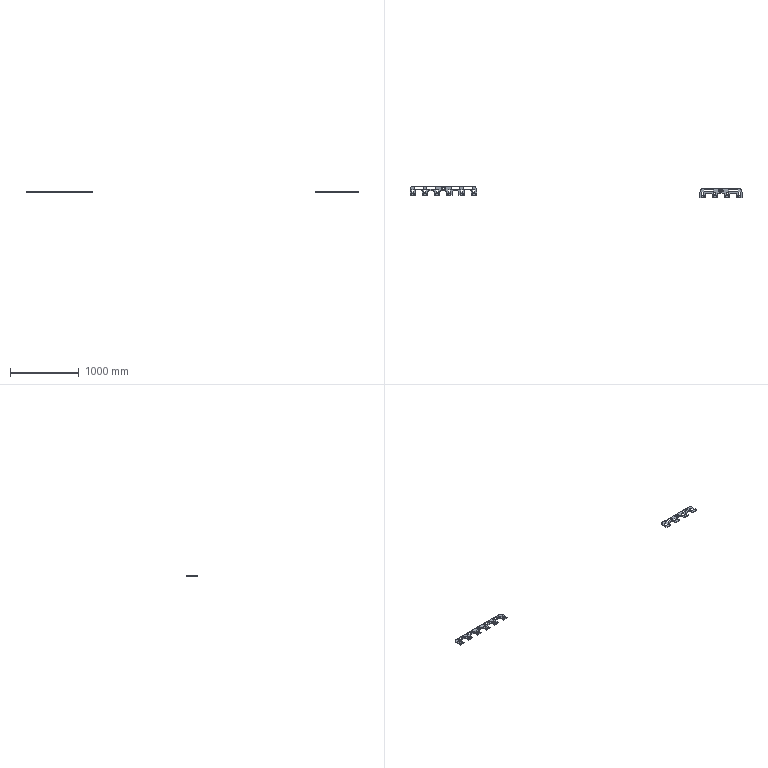NC program | NX | posted with a generic post | part box 4825 x 168.213 x 13 mm
Lines 6552 to 7588 of 14244:
(HOLE_MILLING_COPY , TOOL : D6)
N13054 T06 M6
N13056 G54
N13058 G17 G0 G90 X472.685 Y58.869 S9500 M3
N13060 G43 Z30. H6
N13062 Z0.5
N13064 G94 G3 X473.185 Y58.369 R0.5 F1400.
N13066 X473.685 Y58.869 R0.5
N13068 X473.685 Y58.869 Z0. I-1. J0.
N13070 X473.685 Y58.869 Z-0.5 I-1. J0.
N13072 X473.685 Y58.869 Z-1. I-1. J0.
N13074 X473.685 Y58.869 Z-1.5 I-1. J0.
N13076 X473.685 Y58.869 Z-2. I-1. J0.
N13078 X473.685 Y58.869 Z-2.5 I-1. J0.
N13080 X473.685 Y58.869 Z-3. I-1. J0.
N13082 X473.685 Y58.869 Z-3.5 I-1. J0.
N13084 X473.685 Y58.869 Z-4. I-1. J0.
N13086 X473.685 Y58.869 Z-4.5 I-1. J0.
N13088 X472.994 Y59.82 Z-4.6 R1.
N13090 X471.734 Y59.178 R1.
N13092 X472.994 Y59.82 R-1.
N13094 X472.364 Y59.499 R0.5
N13096 X472.685 Y58.869 R0.5
N13098 G0 Z30.
N13100 X457.531 Y43.715
N13102 Z0.5
N13104 G3 X458.031 Y43.215 R0.5
N13106 X458.531 Y43.715 R0.5
N13108 X458.531 Y43.715 Z0. I-1. J0.
N13110 X458.531 Y43.715 Z-0.5 I-1. J0.
N13112 X458.531 Y43.715 Z-1. I-1. J0.
N13114 X458.531 Y43.715 Z-1.5 I-1. J0.
N13116 X458.531 Y43.715 Z-2. I-1. J0.
N13118 X458.531 Y43.715 Z-2.5 I-1. J0.
N13120 X458.531 Y43.715 Z-3. I-1. J0.
N13122 X458.531 Y43.715 Z-3.5 I-1. J0.
N13124 X458.531 Y43.715 Z-4. I-1. J0.
N13126 X458.531 Y43.715 Z-4.5 I-1. J0.
N13128 X457.84 Y44.666 Z-4.6 R1.
N13130 X456.58 Y44.024 R1.
N13132 X457.84 Y44.666 R-1.
N13134 X457.21 Y44.345 R0.5
N13136 X457.531 Y43.715 R0.5
N13138 G0 Z30.
N13140 Y22.285
N13142 Z0.5
N13144 G3 X458.031 Y21.785 R0.5
N13146 X458.531 Y22.285 R0.5
N13148 X458.531 Y22.285 Z0. I-1. J0.
N13150 X458.531 Y22.285 Z-0.5 I-1. J0.
N13152 X458.531 Y22.285 Z-1. I-1. J0.
N13154 X458.531 Y22.285 Z-1.5 I-1. J0.
N13156 X458.531 Y22.285 Z-2. I-1. J0.
N13158 X458.531 Y22.285 Z-2.5 I-1. J0.
N13160 X458.531 Y22.285 Z-3. I-1. J0.
N13162 X458.531 Y22.285 Z-3.5 I-1. J0.
N13164 X458.531 Y22.285 Z-4. I-1. J0.
N13166 X458.531 Y22.285 Z-4.5 I-1. J0.
N13168 X457.84 Y23.236 Z-4.6 R1.
N13170 X456.58 Y22.594 R1.
N13172 X457.84 Y23.236 R-1.
N13174 X457.21 Y22.915 R0.5
N13176 X457.531 Y22.285 R0.5
N13178 G0 Z30.
N13180 X472.685 Y7.131
N13182 Z0.5
N13184 G3 X473.185 Y6.631 R0.5
N13186 X473.685 Y7.131 R0.5
N13188 X473.685 Y7.131 Z0. I-1. J0.
N13190 X473.685 Y7.131 Z-0.5 I-1. J0.
N13192 X473.685 Y7.131 Z-1. I-1. J0.
N13194 X473.685 Y7.131 Z-1.5 I-1. J0.
N13196 X473.685 Y7.131 Z-2. I-1. J0.
N13198 X473.685 Y7.131 Z-2.5 I-1. J0.
N13200 X473.685 Y7.131 Z-3. I-1. J0.
N13202 X473.685 Y7.131 Z-3.5 I-1. J0.
N13204 X473.685 Y7.131 Z-4. I-1. J0.
N13206 X473.685 Y7.131 Z-4.5 I-1. J0.
N13208 X472.994 Y8.082 Z-4.6 R1.
N13210 X471.734 Y7.44 R1.
N13212 X472.994 Y8.082 R-1.
N13214 X472.364 Y7.761 R0.5
N13216 X472.685 Y7.131 R0.5
N13218 G0 Z30.
N13220 X494.115
N13222 Z0.5
N13224 G3 X494.615 Y6.631 R0.5
N13226 X495.115 Y7.131 R0.5
N13228 X495.115 Y7.131 Z0. I-1. J0.
N13230 X495.115 Y7.131 Z-0.5 I-1. J0.
N13232 X495.115 Y7.131 Z-1. I-1. J0.
N13234 X495.115 Y7.131 Z-1.5 I-1. J0.
N13236 X495.115 Y7.131 Z-2. I-1. J0.
N13238 X495.115 Y7.131 Z-2.5 I-1. J0.
N13240 X495.115 Y7.131 Z-3. I-1. J0.
N13242 X495.115 Y7.131 Z-3.5 I-1. J0.
N13244 X495.115 Y7.131 Z-4. I-1. J0.
N13246 X495.115 Y7.131 Z-4.5 I-1. J0.
N13248 X494.424 Y8.082 Z-4.6 R1.
N13250 X493.164 Y7.44 R1.
N13252 X494.424 Y8.082 R-1.
N13254 X493.794 Y7.761 R0.5
N13256 X494.115 Y7.131 R0.5
N13258 G0 Z30.
N13260 X509.269 Y22.285
N13262 Z0.5
N13264 G3 X509.769 Y21.785 R0.5
N13266 X510.269 Y22.285 R0.5
N13268 X510.269 Y22.285 Z0. I-1. J0.
N13270 X510.269 Y22.285 Z-0.5 I-1. J0.
N13272 X510.269 Y22.285 Z-1. I-1. J0.
N13274 X510.269 Y22.285 Z-1.5 I-1. J0.
N13276 X510.269 Y22.285 Z-2. I-1. J0.
N13278 X510.269 Y22.285 Z-2.5 I-1. J0.
N13280 X510.269 Y22.285 Z-3. I-1. J0.
N13282 X510.269 Y22.285 Z-3.5 I-1. J0.
N13284 X510.269 Y22.285 Z-4. I-1. J0.
N13286 X510.269 Y22.285 Z-4.5 I-1. J0.
N13288 X509.578 Y23.236 Z-4.6 R1.
N13290 X508.318 Y22.594 R1.
N13292 X509.578 Y23.236 R-1.
N13294 X508.948 Y22.915 R0.5
N13296 X509.269 Y22.285 R0.5
N13298 G0 Z30.
N13300 Y43.715
N13302 Z0.5
N13304 G3 X509.769 Y43.215 R0.5
N13306 X510.269 Y43.715 R0.5
N13308 X510.269 Y43.715 Z0. I-1. J0.
N13310 X510.269 Y43.715 Z-0.5 I-1. J0.
N13312 X510.269 Y43.715 Z-1. I-1. J0.
N13314 X510.269 Y43.715 Z-1.5 I-1. J0.
N13316 X510.269 Y43.715 Z-2. I-1. J0.
N13318 X510.269 Y43.715 Z-2.5 I-1. J0.
N13320 X510.269 Y43.715 Z-3. I-1. J0.
N13322 X510.269 Y43.715 Z-3.5 I-1. J0.
N13324 X510.269 Y43.715 Z-4. I-1. J0.
N13326 X510.269 Y43.715 Z-4.5 I-1. J0.
N13328 X509.578 Y44.666 Z-4.6 R1.
N13330 X508.318 Y44.024 R1.
N13332 X509.578 Y44.666 R-1.
N13334 X508.948 Y44.345 R0.5
N13336 X509.269 Y43.715 R0.5
N13338 G0 Z30.
N13340 X494.115 Y58.869
N13342 Z0.5
N13344 G3 X494.615 Y58.369 R0.5
N13346 X495.115 Y58.869 R0.5
N13348 X495.115 Y58.869 Z0. I-1. J0.
N13350 X495.115 Y58.869 Z-0.5 I-1. J0.
N13352 X495.115 Y58.869 Z-1. I-1. J0.
N13354 X495.115 Y58.869 Z-1.5 I-1. J0.
N13356 X495.115 Y58.869 Z-2. I-1. J0.
N13358 X495.115 Y58.869 Z-2.5 I-1. J0.
N13360 X495.115 Y58.869 Z-3. I-1. J0.
N13362 X495.115 Y58.869 Z-3.5 I-1. J0.
N13364 X495.115 Y58.869 Z-4. I-1. J0.
N13366 X495.115 Y58.869 Z-4.5 I-1. J0.
N13368 X494.424 Y59.82 Z-4.6 R1.
N13370 X493.164 Y59.178 R1.
N13372 X494.424 Y59.82 R-1.
N13374 X493.794 Y59.499 R0.5
N13376 X494.115 Y58.869 R0.5
N13378 G0 Z30.
(ZLEVEL_PROFILE_COPY_1_COPY , TOOL : D6)
N13380 X364.221 Y29.2
N13382 Z-0.591
N13384 G1 Y28.003 F1000.
N13386 X364.284 Y28.
N13388 X366.5 F1650.
N13390 Y30.216
N13392 X366.497 Y30.279
N13394 X365.3
N13396 G0 X364.221 Y29.2 Z-1.182
N13398 G1 Y28.003 F1000.
N13400 X364.284 Y28.
N13402 X366.5 F1650.
N13404 Y30.216
N13406 X366.497 Y30.279
N13408 X365.3
N13410 G0 X364.221 Y29.2 Z-1.773
N13412 G1 Y28.003 F1000.
N13414 X364.284 Y28.
N13416 X366.5 F1650.
N13418 Y30.216
N13420 X366.497 Y30.279
N13422 X365.3
N13424 G0 X364.221 Y29.2 Z-2.364
N13426 G1 Y28.003 F1000.
N13428 X364.284 Y28.
N13430 X366.5 F1650.
N13432 Y30.216
N13434 X366.497 Y30.279
N13436 X365.3
N13438 G0 X364.221 Y29.2 Z-2.955
N13440 G1 Y28.003 F1000.
N13442 X364.284 Y28.
N13444 X366.5 F1650.
N13446 Y30.216
N13448 X366.497 Y30.279
N13450 X365.3
N13452 G0 X364.221 Y29.2 Z-3.545
N13454 G1 Y28.003 F1000.
N13456 X364.284 Y28.
N13458 X366.5 F1650.
N13460 Y30.216
N13462 X366.497 Y30.279
N13464 X365.3
N13466 G0 X364.221 Y29.2 Z-4.136
N13468 G1 Y28.003 F1000.
N13470 X364.284 Y28.
N13472 X366.5 F1650.
N13474 Y30.216
N13476 X366.497 Y30.279
N13478 X365.3
N13480 G0 X364.221 Y29.2 Z-4.727
N13482 G1 Y28.003 F1000.
N13484 X364.284 Y28.
N13486 X366.5 F1650.
N13488 Y30.216
N13490 X366.497 Y30.279
N13492 X365.3
N13494 G0 X364.221 Y29.2 Z-5.318
N13496 G1 Y28.003 F1000.
N13498 X364.284 Y28.
N13500 X366.5 F1650.
N13502 Y30.216
N13504 X366.497 Y30.279
N13506 X365.3
N13508 G0 X364.221 Y29.2 Z-5.909
N13510 G1 Y28.003 F1000.
N13512 X364.284 Y28.
N13514 X366.5 F1650.
N13516 Y30.216
N13518 X366.497 Y30.279
N13520 X365.3
N13522 G0 X364.221 Y29.2 Z-6.5
N13524 G1 Y28.003 F1000.
N13526 X364.284 Y28.
N13528 X366.5 F1650.
N13530 Y30.216
N13532 X366.497 Y30.279
N13534 X365.3
N13536 G0 X364.221 Y29.2 Z-7.091
N13538 G1 Y28.003 F1000.
N13540 X364.284 Y28.
N13542 X366.5 F1650.
N13544 Y30.216
N13546 X366.497 Y30.279
N13548 X365.3
N13550 G0 X364.221 Y29.2 Z-7.682
N13552 G1 Y28.003 F1000.
N13554 X364.284 Y28.
N13556 X366.5 F1650.
N13558 Y30.216
N13560 X366.497 Y30.279
N13562 X365.3
N13564 G0 X364.221 Y29.2 Z-8.273
N13566 G1 Y28.003 F1000.
N13568 X364.284 Y28.
N13570 X366.5 F1650.
N13572 Y30.216
N13574 X366.497 Y30.279
N13576 X365.3
N13578 G0 X364.221 Y29.2 Z-8.864
N13580 G1 Y28.003 F1000.
N13582 X364.284 Y28.
N13584 X366.5 F1650.
N13586 Y30.216
N13588 X366.497 Y30.279
N13590 X365.3
N13592 G0 X364.221 Y29.2 Z-9.455
N13594 G1 Y28.003 F1000.
N13596 X364.284 Y28.
N13598 X366.5 F1650.
N13600 Y30.216
N13602 X366.497 Y30.279
N13604 X365.3
N13606 G0 X364.221 Y29.2 Z-10.045
N13608 G1 Y28.003 F1000.
N13610 X364.284 Y28.
N13612 X366.5 F1650.
N13614 Y30.216
N13616 X366.497 Y30.279
N13618 X365.3
N13620 G0 X364.221 Y29.2 Z-10.636
N13622 G1 Y28.003 F1000.
N13624 X364.284 Y28.
N13626 X366.5 F1650.
N13628 Y30.216
N13630 X366.497 Y30.279
N13632 X365.3
N13634 G0 X364.221 Y29.2 Z-11.227
N13636 G1 Y28.003 F1000.
N13638 X364.284 Y28.
N13640 X366.5 F1650.
N13642 Y30.216
N13644 X366.497 Y30.279
N13646 X365.3
N13648 G0 X364.221 Y29.2 Z-11.818
N13650 G1 Y28.003 F1000.
N13652 X364.284 Y28.
N13654 X366.5 F1650.
N13656 Y30.216
N13658 X366.497 Y30.279
N13660 X365.3
N13662 G0 X364.221 Y29.2 Z-12.409
N13664 G1 Y28.003 F1000.
N13666 X364.284 Y28.
N13668 X366.5 F1650.
N13670 Y30.216
N13672 X366.497 Y30.279
N13674 X365.3
N13676 G0 X364.221 Y29.2 Z-13.
N13678 G1 Y28.003 F1000.
N13680 X364.284 Y28.
N13682 X366.5 F1650.
N13684 Y30.216
N13686 X366.497 Y30.279
N13688 X365.3
N13690 G0 Z30.
N13692 Y51.721
N13694 Z-0.591
N13696 G1 X366.497 F1000.
N13698 X366.5 Y51.784
N13700 Y54. F1650.
N13702 X364.284
N13704 X364.221 Y53.997
N13706 Y52.8
N13708 G0 X365.3 Y51.721 Z-1.182
N13710 G1 X366.497 F1000.
N13712 X366.5 Y51.784
N13714 Y54. F1650.
N13716 X364.284
N13718 X364.221 Y53.997
N13720 Y52.8
N13722 G0 X365.3 Y51.721 Z-1.773
N13724 G1 X366.497 F1000.
N13726 X366.5 Y51.784
N13728 Y54. F1650.
N13730 X364.284
N13732 X364.221 Y53.997
N13734 Y52.8
N13736 G0 X365.3 Y51.721 Z-2.364
N13738 G1 X366.497 F1000.
N13740 X366.5 Y51.784
N13742 Y54. F1650.
N13744 X364.284
N13746 X364.221 Y53.997
N13748 Y52.8
N13750 G0 X365.3 Y51.721 Z-2.955
N13752 G1 X366.497 F1000.
N13754 X366.5 Y51.784
N13756 Y54. F1650.
N13758 X364.284
N13760 X364.221 Y53.997
N13762 Y52.8
N13764 G0 X365.3 Y51.721 Z-3.545
N13766 G1 X366.497 F1000.
N13768 X366.5 Y51.784
N13770 Y54. F1650.
N13772 X364.284
N13774 X364.221 Y53.997
N13776 Y52.8
N13778 G0 X365.3 Y51.721 Z-4.136
N13780 G1 X366.497 F1000.
N13782 X366.5 Y51.784
N13784 Y54. F1650.
N13786 X364.284
N13788 X364.221 Y53.997
N13790 Y52.8
N13792 G0 X365.3 Y51.721 Z-4.727
N13794 G1 X366.497 F1000.
N13796 X366.5 Y51.784
N13798 Y54. F1650.
N13800 X364.284
N13802 X364.221 Y53.997
N13804 Y52.8
N13806 G0 X365.3 Y51.721 Z-5.318
N13808 G1 X366.497 F1000.
N13810 X366.5 Y51.784
N13812 Y54. F1650.
N13814 X364.284
N13816 X364.221 Y53.997
N13818 Y52.8
N13820 G0 X365.3 Y51.721 Z-5.909
N13822 G1 X366.497 F1000.
N13824 X366.5 Y51.784
N13826 Y54. F1650.
N13828 X364.284
N13830 X364.221 Y53.997
N13832 Y52.8
N13834 G0 X365.3 Y51.721 Z-6.5
N13836 G1 X366.497 F1000.
N13838 X366.5 Y51.784
N13840 Y54. F1650.
N13842 X364.284
N13844 X364.221 Y53.997
N13846 Y52.8
N13848 G0 X365.3 Y51.721 Z-7.091
N13850 G1 X366.497 F1000.
N13852 X366.5 Y51.784
N13854 Y54. F1650.
N13856 X364.284
N13858 X364.221 Y53.997
N13860 Y52.8
N13862 G0 X365.3 Y51.721 Z-7.682
N13864 G1 X366.497 F1000.
N13866 X366.5 Y51.784
N13868 Y54. F1650.
N13870 X364.284
N13872 X364.221 Y53.997
N13874 Y52.8
N13876 G0 X365.3 Y51.724 Z-8.273
N13878 G1 X366.497 F1000.
N13880 X366.5 Y51.787
N13882 Y53.99 F1650.
N13884 Y54.
N13886 X364.295
N13888 X364.232 Y53.997
N13890 Y52.8
N13892 G0 X365.3 Y51.724 Z-8.864
N13894 G1 X366.497 F1000.
N13896 X366.5 Y51.787
N13898 Y53.99 F1650.
N13900 Y54.
N13902 X364.295
N13904 X364.232 Y53.997
N13906 Y52.8
N13908 G0 X365.3 Y51.724 Z-9.455
N13910 G1 X366.497 F1000.
N13912 X366.5 Y51.787
N13914 Y53.99 F1650.
N13916 Y54.
N13918 X364.295
N13920 X364.232 Y53.997
N13922 Y52.8
N13924 G0 X365.3 Y51.724 Z-10.045
N13926 G1 X366.497 F1000.
N13928 X366.5 Y51.787
N13930 Y53.99 F1650.
N13932 Y54.
N13934 X364.295
N13936 X364.232 Y53.997
N13938 Y52.8
N13940 G0 X365.3 Y51.724 Z-10.636
N13942 G1 X366.497 F1000.
N13944 X366.5 Y51.787
N13946 Y53.99 F1650.
N13948 Y54.
N13950 X364.295
N13952 X364.232 Y53.997
N13954 Y52.8
N13956 G0 X365.3 Y51.724 Z-11.227
N13958 G1 X366.497 F1000.
N13960 X366.5 Y51.787
N13962 Y53.99 F1650.
N13964 Y54.
N13966 X364.295
N13968 X364.232 Y53.997
N13970 Y52.8
N13972 G0 X365.3 Y51.724 Z-11.818
N13974 G1 X366.497 F1000.
N13976 X366.5 Y51.787
N13978 Y53.99 F1650.
N13980 Y54.
N13982 X364.295
N13984 X364.232 Y53.997
N13986 Y52.8
N13988 G0 X365.3 Y51.724 Z-12.409
N13990 G1 X366.497 F1000.
N13992 X366.5 Y51.787
N13994 Y53.99 F1650.
N13996 Y54.
N13998 X364.295
N14000 X364.232 Y53.997
N14002 Y52.8
N14004 G0 X365.3 Y51.724 Z-13.
N14006 G1 X366.497 F1000.
N14008 X366.5 Y51.787
N14010 Y53.99 F1650.
N14012 Y54.
N14014 X364.295
N14016 X364.232 Y53.997
N14018 Y52.8
N14020 G0 Z30.
N14022 X246.979
N14024 Z-0.591
N14026 G1 Y53.997 F1000.
N14028 X246.916 Y54.
N14030 X244.7 F1650.
N14032 Y51.784
N14034 X244.703 Y51.721
N14036 X245.9
N14038 G0 X246.979 Y52.8 Z-1.182
N14040 G1 Y53.997 F1000.
N14042 X246.916 Y54.
N14044 X244.7 F1650.
N14046 Y51.784
N14048 X244.703 Y51.721
N14050 X245.9
N14052 G0 X246.979 Y52.8 Z-1.773
N14054 G1 Y53.997 F1000.
N14056 X246.916 Y54.
N14058 X244.7 F1650.
N14060 Y51.784
N14062 X244.703 Y51.721
N14064 X245.9
N14066 G0 X246.979 Y52.8 Z-2.364
N14068 G1 Y53.997 F1000.
N14070 X246.916 Y54.
N14072 X244.7 F1650.
N14074 Y51.784
N14076 X244.703 Y51.721
N14078 X245.9
N14080 G0 X246.979 Y52.8 Z-2.955
N14082 G1 Y53.997 F1000.
N14084 X246.916 Y54.
N14086 X244.7 F1650.
N14088 Y51.784
N14090 X244.703 Y51.721
N14092 X245.9
N14094 G0 X246.979 Y52.8 Z-3.545
N14096 G1 Y53.997 F1000.
N14098 X246.916 Y54.
N14100 X244.7 F1650.
N14102 Y51.784
N14104 X244.703 Y51.721
N14106 X245.9
N14108 G0 X246.979 Y52.8 Z-4.136
N14110 G1 Y53.997 F1000.
N14112 X246.916 Y54.
N14114 X244.7 F1650.
N14116 Y51.784
N14118 X244.703 Y51.721
N14120 X245.9
N14122 G0 X246.979 Y52.8 Z-4.727
N14124 G1 Y53.997 F1000.
N14126 X246.916 Y54.
N14128 X244.7 F1650.
N14130 Y51.784
N14132 X244.703 Y51.721
N14134 X245.9
N14136 G0 X246.979 Y52.8 Z-5.318
N14138 G1 Y53.997 F1000.
N14140 X246.916 Y54.
N14142 X244.7 F1650.
N14144 Y51.784
N14146 X244.703 Y51.721
N14148 X245.9
N14150 G0 X246.979 Y52.8 Z-5.909
N14152 G1 Y53.997 F1000.
N14154 X246.916 Y54.
N14156 X244.7 F1650.
N14158 Y51.784
N14160 X244.703 Y51.721
N14162 X245.9
N14164 G0 X246.979 Y52.8 Z-6.5
N14166 G1 Y53.997 F1000.
N14168 X246.916 Y54.
N14170 X244.7 F1650.
N14172 Y51.784
N14174 X244.703 Y51.721
N14176 X245.9
N14178 G0 X246.979 Y52.8 Z-7.091
N14180 G1 Y53.997 F1000.
N14182 X246.916 Y54.
N14184 X244.7 F1650.
N14186 Y51.784
N14188 X244.703 Y51.721
N14190 X245.9
N14192 G0 X246.979 Y52.8 Z-7.682
N14194 G1 Y53.997 F1000.
N14196 X246.916 Y54.
N14198 X244.7 F1650.
N14200 Y51.784
N14202 X244.703 Y51.721
N14204 X245.9
N14206 G0 X246.969 Y52.8 Z-8.273
N14208 G1 Y53.997 F1000.
N14210 X246.906 Y54.
N14212 X244.7 F1650.
N14214 Y51.787
N14216 X244.703 Y51.725
N14218 X245.9
N14220 G0 X246.969 Y52.8 Z-8.864
N14222 G1 Y53.997 F1000.
N14224 X246.906 Y54.
N14226 X244.7 F1650.
N14228 Y51.787
N14230 X244.703 Y51.725
N14232 X245.9
N14234 G0 X246.969 Y52.8 Z-9.455
N14236 G1 Y53.997 F1000.
N14238 X246.906 Y54.
N14240 X244.7 F1650.
N14242 Y51.787
N14244 X244.703 Y51.725
N14246 X245.9
N14248 G0 X246.969 Y52.8 Z-10.045
N14250 G1 Y53.997 F1000.
N14252 X246.906 Y54.
N14254 X244.7 F1650.
N14256 Y51.787
N14258 X244.703 Y51.725
N14260 X245.9
N14262 G0 X246.969 Y52.8 Z-10.636
N14264 G1 Y53.997 F1000.
N14266 X246.906 Y54.
N14268 X244.7 F1650.
N14270 Y51.787
N14272 X244.703 Y51.725
N14274 X245.9
N14276 G0 X246.969 Y52.8 Z-11.227
N14278 G1 Y53.997 F1000.
N14280 X246.906 Y54.
N14282 X244.7 F1650.
N14284 Y51.787
N14286 X244.703 Y51.725
N14288 X245.9
N14290 G0 X246.969 Y52.8 Z-11.818
N14292 G1 Y53.997 F1000.
N14294 X246.906 Y54.
N14296 X244.7 F1650.
N14298 Y51.787
N14300 X244.703 Y51.725
N14302 X245.9
N14304 G0 X246.969 Y52.8 Z-12.409
N14306 G1 Y53.997 F1000.
N14308 X246.906 Y54.
N14310 X244.7 F1650.
N14312 Y51.787
N14314 X244.703 Y51.725
N14316 X245.9
N14318 G0 X246.969 Y52.8 Z-13.
N14320 G1 Y53.997 F1000.
N14322 X246.906 Y54.
N14324 X244.7 F1650.
N14326 Y51.787
N14328 X244.703 Y51.725
N14330 X245.9
N14332 G0 Z30.
N14334 Y30.279
N14336 Z-0.591
N14338 G1 X244.703 F1000.
N14340 X244.7 Y30.216
N14342 Y28.065 F1650.
N14344 X244.699 Y27.999
N14346 X244.714 Y28.
N14348 X246.916
N14350 X246.979 Y28.003
N14352 Y29.2
N14354 G0 X245.9 Y30.279 Z-1.182
N14356 G1 X244.703 F1000.
N14358 X244.7 Y30.216
N14360 Y28.065 F1650.
N14362 X244.699 Y27.999
N14364 X244.714 Y28.
N14366 X246.916
N14368 X246.979 Y28.003
N14370 Y29.2
N14372 G0 X245.9 Y30.279 Z-1.773
N14374 G1 X244.703 F1000.
N14376 X244.7 Y30.216
N14378 Y28.065 F1650.
N14380 X244.699 Y27.999
N14382 X244.714 Y28.
N14384 X246.916
N14386 X246.979 Y28.003
N14388 Y29.2
N14390 G0 X245.9 Y30.279 Z-2.364
N14392 G1 X244.703 F1000.
N14394 X244.7 Y30.216
N14396 Y28.065 F1650.
N14398 X244.699 Y27.999
N14400 X244.714 Y28.
N14402 X246.916
N14404 X246.979 Y28.003
N14406 Y29.2
N14408 G0 X245.9 Y30.279 Z-2.955
N14410 G1 X244.703 F1000.
N14412 X244.7 Y30.216
N14414 Y28.065 F1650.
N14416 X244.699 Y27.999
N14418 X246.916 Y28.
N14420 X246.979 Y28.003
N14422 Y29.2
N14424 G0 X245.9 Y30.279 Z-3.545
N14426 G1 X244.703 F1000.
N14428 X244.7 Y30.216
N14430 Y28.065 F1650.
N14432 X244.699 Y27.999
N14434 X246.916 Y28.
N14436 X246.979 Y28.003
N14438 Y29.2
N14440 G0 X245.9 Y30.279 Z-4.136
N14442 G1 X244.703 F1000.
N14444 X244.7 Y30.216
N14446 Y28.065 F1650.
N14448 X244.699 Y27.999
N14450 X246.916 Y28.
N14452 X246.979 Y28.003
N14454 Y29.2
N14456 G0 X245.9 Y30.279 Z-4.727
N14458 G1 X244.703 F1000.
N14460 X244.7 Y30.216
N14462 Y28.065 F1650.
N14464 X244.699 Y27.999
N14466 X246.916 Y28.
N14468 X246.979 Y28.003
N14470 Y29.2
N14472 G0 X245.9 Y30.279 Z-5.318
N14474 G1 X244.703 F1000.
N14476 X244.7 Y30.216
N14478 Y28.065 F1650.
N14480 Y28.
N14482 X246.916
N14484 X246.979 Y28.003
N14486 Y29.2
N14488 G0 X245.9 Y30.279 Z-5.909
N14490 G1 X244.703 F1000.
N14492 X244.7 Y30.216
N14494 Y28.065 F1650.
N14496 Y28.
N14498 X246.916
N14500 X246.979 Y28.003
N14502 Y29.2
N14504 G0 X245.9 Y30.279 Z-6.5
N14506 G1 X244.703 F1000.
N14508 X244.7 Y30.216
N14510 Y28.065 F1650.
N14512 Y28.
N14514 X246.916
N14516 X246.979 Y28.003
N14518 Y29.2
N14520 G0 X245.9 Y30.279 Z-7.091
N14522 G1 X244.703 F1000.
N14524 X244.7 Y30.216
N14526 Y28. F1650.
N14528 X246.916
N14530 X246.979 Y28.003
N14532 Y29.2
N14534 G0 X245.9 Y30.279 Z-7.682
N14536 G1 X244.703 F1000.
N14538 X244.7 Y30.216
N14540 Y28.04 F1650.
N14542 Y28.
N14544 X246.916
N14546 X246.979 Y28.003
N14548 Y29.2
N14550 G0 X245.9 Y30.279 Z-8.273
N14552 G1 X244.703 F1000.
N14554 X244.7 Y30.217
N14556 Y28. F1650.
N14558 X246.918
N14560 X246.98 Y28.003
N14562 Y29.2
N14564 G0 X245.9 Y30.279 Z-8.864
N14566 G1 X244.703 F1000.
N14568 X244.7 Y30.217
N14570 Y28. F1650.
N14572 X246.918
N14574 X246.98 Y28.003
N14576 Y29.2
N14578 G0 X245.9 Y30.279 Z-9.455
N14580 G1 X244.703 F1000.
N14582 X244.7 Y30.217
N14584 Y28. F1650.
N14586 X246.918
N14588 X246.98 Y28.003
N14590 Y29.2
N14592 G0 X245.9 Y30.279 Z-10.045
N14594 G1 X244.703 F1000.
N14596 X244.7 Y30.217
N14598 Y28. F1650.
N14600 X246.918
N14602 X246.98 Y28.003
N14604 Y29.2
N14606 G0 X245.9 Y30.279 Z-10.636
N14608 G1 X244.703 F1000.
N14610 X244.7 Y30.217
N14612 Y28. F1650.
N14614 X246.918
N14616 X246.98 Y28.003
N14618 Y29.2
N14620 G0 X245.9 Y30.279 Z-11.227
N14622 G1 X244.703 F1000.
N14624 X244.7 Y30.217
N14626 Y28. F1650.
N14628 X246.918
N14630 X246.98 Y28.003
N14632 Y29.2
N14634 G0 X245.9 Y30.279 Z-11.818
N14636 G1 X244.703 F1000.
N14638 X244.7 Y30.217
N14640 Y28. F1650.
N14642 X246.918
N14644 X246.98 Y28.003
N14646 Y29.2
N14648 G0 X245.9 Y30.279 Z-12.409
N14650 G1 X244.703 F1000.
N14652 X244.7 Y30.217
N14654 Y28. F1650.
N14656 X246.918
N14658 X246.98 Y28.003
N14660 Y29.2
N14662 G0 X245.9 Y30.279 Z-13.
N14664 G1 X244.703 F1000.
N14666 X244.7 Y30.217
N14668 Y28. F1650.
N14670 X246.918
N14672 X246.98 Y28.003
N14674 Y29.2
N14676 G0 Z30.
N14678 X186.421
N14680 Z-0.591
N14682 G1 Y28.003 F1000.
N14684 X186.484 Y28.
N14686 X188.7 F1650.
N14688 Y30.216
N14690 X188.697 Y30.279
N14692 X187.5
N14694 G0 X186.421 Y29.2 Z-1.182
N14696 G1 Y28.003 F1000.
N14698 X186.484 Y28.
N14700 X188.7 F1650.
N14702 Y30.216
N14704 X188.697 Y30.279
N14706 X187.5
N14708 G0 X186.421 Y29.2 Z-1.773
N14710 G1 Y28.003 F1000.
N14712 X186.484 Y28.
N14714 X188.7 F1650.
N14716 Y30.216
N14718 X188.697 Y30.279
N14720 X187.5
N14722 G0 X186.421 Y29.2 Z-2.364
N14724 G1 Y28.003 F1000.
N14726 X186.484 Y28.
N14728 X188.7 F1650.
N14730 Y30.216
N14732 X188.697 Y30.279
N14734 X187.5
N14736 G0 X186.421 Y29.2 Z-2.955
N14738 G1 Y28.003 F1000.
N14740 X186.484 Y28.
N14742 X188.7 F1650.
N14744 Y30.216
N14746 X188.697 Y30.279
N14748 X187.5
N14750 G0 X186.421 Y29.2 Z-3.545
N14752 G1 Y28.003 F1000.
N14754 X186.484 Y28.
N14756 X188.7 F1650.
N14758 Y30.216
N14760 X188.697 Y30.279
N14762 X187.5
N14764 G0 X186.421 Y29.2 Z-4.136
N14766 G1 Y28.003 F1000.
N14768 X186.484 Y28.
N14770 X188.7 F1650.
N14772 Y30.216
N14774 X188.697 Y30.279
N14776 X187.5
N14778 G0 X186.421 Y29.2 Z-4.727
N14780 G1 Y28.003 F1000.
N14782 X186.484 Y28.
N14784 X188.7 F1650.
N14786 Y30.216
N14788 X188.697 Y30.279
N14790 X187.5
N14792 G0 X186.421 Y29.2 Z-5.318
N14794 G1 Y28.003 F1000.
N14796 X186.484 Y28.
N14798 X188.7 F1650.
N14800 Y30.216
N14802 X188.697 Y30.279
N14804 X187.5
N14806 G0 X186.421 Y29.2 Z-5.909
N14808 G1 Y28.003 F1000.
N14810 X186.484 Y28.
N14812 X188.7 F1650.
N14814 Y30.216
N14816 X188.697 Y30.279
N14818 X187.5
N14820 G0 X186.421 Y29.2 Z-6.5
N14822 G1 Y28.003 F1000.
N14824 X186.484 Y28.
N14826 X188.7 F1650.
N14828 Y30.216
N14830 X188.697 Y30.279
N14832 X187.5
N14834 G0 X186.421 Y29.2 Z-7.091
N14836 G1 Y28.003 F1000.
N14838 X186.484 Y28.
N14840 X188.7 F1650.
N14842 Y30.216
N14844 X188.697 Y30.279
N14846 X187.5
N14848 G0 X186.421 Y29.2 Z-7.682
N14850 G1 Y28.003 F1000.
N14852 X186.484 Y28.
N14854 X188.7 F1650.
N14856 Y30.216
N14858 X188.697 Y30.279
N14860 X187.5
N14862 G0 X186.416 Y29.2 Z-8.273
N14864 G1 Y28.003 F1000.
N14866 X186.479 Y28.
N14868 X188.7 F1650.
N14870 Y30.217
N14872 X188.697 Y30.28
N14874 X187.5
N14876 G0 X186.416 Y29.2 Z-8.864
N14878 G1 Y28.003 F1000.
N14880 X186.479 Y28.
N14882 X188.7 F1650.
N14884 Y30.217
N14886 X188.697 Y30.28
N14888 X187.5
N14890 G0 X186.416 Y29.2 Z-9.455
N14892 G1 Y28.003 F1000.
N14894 X186.479 Y28.
N14896 X188.7 F1650.
N14898 Y30.217
N14900 X188.697 Y30.28
N14902 X187.5
N14904 G0 X186.416 Y29.2 Z-10.045
N14906 G1 Y28.003 F1000.
N14908 X186.479 Y28.
N14910 X188.7 F1650.
N14912 Y30.217
N14914 X188.697 Y30.28
N14916 X187.5
N14918 G0 X186.416 Y29.2 Z-10.636
N14920 G1 Y28.003 F1000.
N14922 X186.479 Y28.
N14924 X188.7 F1650.
N14926 Y30.217
N14928 X188.697 Y30.28
N14930 X187.5
N14932 G0 X186.416 Y29.2 Z-11.227
N14934 G1 Y28.003 F1000.
N14936 X186.479 Y28.
N14938 X188.7 F1650.
N14940 Y30.217
N14942 X188.697 Y30.28
N14944 X187.5
N14946 G0 X186.416 Y29.2 Z-11.818
N14948 G1 Y28.003 F1000.
N14950 X186.479 Y28.
N14952 X188.7 F1650.
N14954 Y30.217
N14956 X188.697 Y30.28
N14958 X187.5
N14960 G0 X186.416 Y29.2 Z-12.409
N14962 G1 Y28.003 F1000.
N14964 X186.479 Y28.
N14966 X188.7 F1650.
N14968 Y30.217
N14970 X188.697 Y30.28
N14972 X187.5
N14974 G0 X186.416 Y29.2 Z-13.
N14976 G1 Y28.003 F1000.
N14978 X186.479 Y28.
N14980 X188.7 F1650.
N14982 Y30.217
N14984 X188.697 Y30.28
N14986 X187.5
N14988 G0 Z30.
N14990 Y51.721
N14992 Z-0.591
N14994 G1 X188.697 F1000.
N14996 X188.7 Y51.784
N14998 Y54. F1650.
N15000 X186.484
N15002 X186.421 Y53.997
N15004 Y52.8
N15006 G0 X187.5 Y51.721 Z-1.182
N15008 G1 X188.697 F1000.
N15010 X188.7 Y51.784
N15012 Y54. F1650.
N15014 X186.484
N15016 X186.421 Y53.997
N15018 Y52.8
N15020 G0 X187.5 Y51.721 Z-1.773
N15022 G1 X188.697 F1000.
N15024 X188.7 Y51.784
N15026 Y54. F1650.
N15028 X186.484
N15030 X186.421 Y53.997
N15032 Y52.8
N15034 G0 X187.5 Y51.721 Z-2.364
N15036 G1 X188.697 F1000.
N15038 X188.7 Y51.784
N15040 Y54. F1650.
N15042 X186.484
N15044 X186.421 Y53.997
N15046 Y52.8
N15048 G0 X187.5 Y51.721 Z-2.955
N15050 G1 X188.697 F1000.
N15052 X188.7 Y51.784
N15054 Y54. F1650.
N15056 X186.484
N15058 X186.421 Y53.997
N15060 Y52.8
N15062 G0 X187.5 Y51.721 Z-3.545
N15064 G1 X188.697 F1000.
N15066 X188.7 Y51.784
N15068 Y54. F1650.
N15070 X186.484
N15072 X186.421 Y53.997
N15074 Y52.8
N15076 G0 X187.5 Y51.721 Z-4.136
N15078 G1 X188.697 F1000.
N15080 X188.7 Y51.784
N15082 Y54. F1650.
N15084 X186.484
N15086 X186.421 Y53.997
N15088 Y52.8
N15090 G0 X187.5 Y51.721 Z-4.727
N15092 G1 X188.697 F1000.
N15094 X188.7 Y51.784
N15096 Y54. F1650.
N15098 X186.484
N15100 X186.421 Y53.997
N15102 Y52.8
N15104 G0 X187.5 Y51.721 Z-5.318
N15106 G1 X188.697 F1000.
N15108 X188.7 Y51.784
N15110 Y54. F1650.
N15112 X186.484
N15114 X186.421 Y53.997